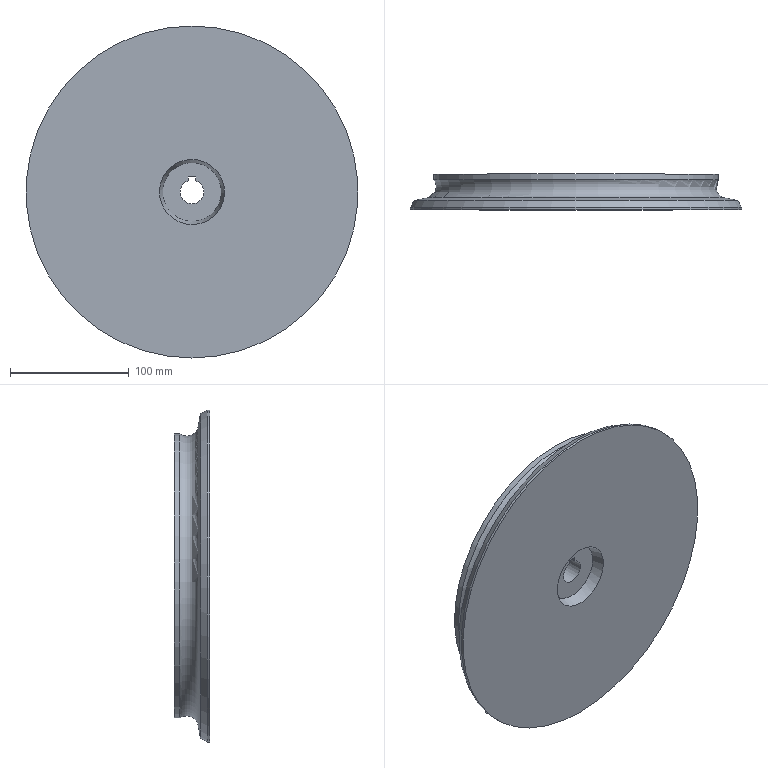Part | NX | features DATUM_CSYS 5, SKETCH 4, EXTRUDE 3, CPROJ 1, Delete Body 1, HOLE PACKAGE 1, SIMPLE HOLE 1, SWP104 1 | 1 solid | 13 faces | box 280 x 30 x 280 mm | volume 1461901 mm3 | plane 6 | cylinder 3 | cone 3 | torus 1 | commonest cylinder face diameters 20 x1 240.085 x1 280 x1
STEP:
#1=CARTESIAN_POINT('',(-3.,31.,151.135));
#2=VERTEX_POINT('',#1);
#3=CARTESIAN_POINT('',(-3.,31.,154.395));
#4=VERTEX_POINT('',#3);
#5=CARTESIAN_POINT('',(-3.,31.,141.595));
#6=DIRECTION('',(0.,0.,1.));
#7=VECTOR('',#6,1000.);
#8=LINE('',#5,#7);
#9=EDGE_CURVE('',#2,#4,#8,.T.);
#10=ORIENTED_EDGE('',*,*,#9,.F.);
#11=CARTESIAN_POINT('',(3.,31.,151.135));
#12=VERTEX_POINT('',#11);
#13=CARTESIAN_POINT('',(0.,31.,141.595));
#14=DIRECTION('',(0.,1.,0.));
#15=DIRECTION('',(0.,0.,1.));
#16=AXIS2_PLACEMENT_3D('',#13,#14,#15);
#17=CIRCLE('',#16,10.);
#18=EDGE_CURVE('',#12,#2,#17,.T.);
#19=ORIENTED_EDGE('',*,*,#18,.F.);
#20=CARTESIAN_POINT('',(3.,31.,154.395));
#21=VERTEX_POINT('',#20);
#22=CARTESIAN_POINT('',(3.,31.,141.595));
#23=DIRECTION('',(0.,0.,-1.));
#24=VECTOR('',#23,1000.);
#25=LINE('',#22,#24);
#26=EDGE_CURVE('',#21,#12,#25,.T.);
#27=ORIENTED_EDGE('',*,*,#26,.F.);
#28=CARTESIAN_POINT('',(0.,31.,154.395));
#29=DIRECTION('',(1.,0.,0.));
#30=VECTOR('',#29,1000.);
#31=LINE('',#28,#30);
#32=EDGE_CURVE('',#4,#21,#31,.T.);
#33=ORIENTED_EDGE('',*,*,#32,.F.);
#34=EDGE_LOOP('',(#10,#19,#27,#33));
#35=FACE_BOUND('',#34,.T.);
#36=CARTESIAN_POINT('',(0.,31.,261.638));
#37=VERTEX_POINT('',#36);
#38=CARTESIAN_POINT('',(0.,31.,141.595));
#39=DIRECTION('',(0.,1.,0.));
#40=DIRECTION('',(0.,0.,1.));
#41=AXIS2_PLACEMENT_3D('',#38,#39,#40);
#42=CIRCLE('',#41,120.043);
#43=EDGE_CURVE('',#37,#37,#42,.T.);
#44=ORIENTED_EDGE('',*,*,#43,.T.);
#45=EDGE_LOOP('',(#44));
#46=FACE_BOUND('',#45,.T.);
#47=CARTESIAN_POINT('',(0.,31.,141.595));
#48=DIRECTION('',(0.,1.,0.));
#49=DIRECTION('',(0.,0.,1.));
#50=AXIS2_PLACEMENT_3D('',#47,#48,#49);
#51=PLANE('',#50);
#52=ADVANCED_FACE('',(#35,#46),#51,.T.);
#53=CARTESIAN_POINT('',(27.473,1.,140.371));
#54=VERTEX_POINT('',#53);
#55=CARTESIAN_POINT('',(0.,1.,141.595));
#56=DIRECTION('',(0.,-1.,0.));
#57=DIRECTION('',(0.999,0.,-0.04452));
#58=AXIS2_PLACEMENT_3D('',#55,#56,#57);
#59=CIRCLE('',#58,27.5);
#60=EDGE_CURVE('',#54,#54,#59,.T.);
#61=ORIENTED_EDGE('',*,*,#60,.F.);
#62=EDGE_LOOP('',(#61));
#63=FACE_BOUND('',#62,.T.);
#64=CARTESIAN_POINT('',(0.,1.,281.595));
#65=VERTEX_POINT('',#64);
#66=CARTESIAN_POINT('',(0.,1.,141.595));
#67=DIRECTION('',(0.,1.,0.));
#68=DIRECTION('',(0.,0.,1.));
#69=AXIS2_PLACEMENT_3D('',#66,#67,#68);
#70=CIRCLE('',#69,140.);
#71=EDGE_CURVE('',#65,#65,#70,.T.);
#72=ORIENTED_EDGE('',*,*,#71,.F.);
#73=EDGE_LOOP('',(#72));
#74=FACE_BOUND('',#73,.T.);
#75=CARTESIAN_POINT('',(0.,1.,141.595));
#76=DIRECTION('',(0.,1.,0.));
#77=DIRECTION('',(0.,0.,1.));
#78=AXIS2_PLACEMENT_3D('',#75,#76,#77);
#79=PLANE('',#78);
#80=ADVANCED_FACE('',(#63,#74),#79,.F.);
#81=ORIENTED_EDGE('',*,*,#71,.T.);
#82=EDGE_LOOP('',(#81));
#83=FACE_BOUND('',#82,.T.);
#84=CARTESIAN_POINT('',(0.,3.,281.595));
#85=VERTEX_POINT('',#84);
#86=CARTESIAN_POINT('',(0.,3.,141.595));
#87=DIRECTION('',(0.,1.,0.));
#88=DIRECTION('',(0.,0.,1.));
#89=AXIS2_PLACEMENT_3D('',#86,#87,#88);
#90=CIRCLE('',#89,140.);
#91=EDGE_CURVE('',#85,#85,#90,.T.);
#92=ORIENTED_EDGE('',*,*,#91,.F.);
#93=EDGE_LOOP('',(#92));
#94=FACE_BOUND('',#93,.T.);
#95=CARTESIAN_POINT('',(0.,106.,141.595));
#96=DIRECTION('',(0.,1.,0.));
#97=DIRECTION('',(0.,0.,1.));
#98=AXIS2_PLACEMENT_3D('',#95,#96,#97);
#99=CYLINDRICAL_SURFACE('',#98,140.);
#100=ADVANCED_FACE('',(#83,#94),#99,.T.);
#101=ORIENTED_EDGE('',*,*,#91,.T.);
#102=EDGE_LOOP('',(#101));
#103=FACE_BOUND('',#102,.T.);
#104=CARTESIAN_POINT('',(0.,8.757,278.534));
#105=VERTEX_POINT('',#104);
#106=CARTESIAN_POINT('',(0.,8.757,141.595));
#107=DIRECTION('',(0.,1.,0.));
#108=DIRECTION('',(0.,0.,1.));
#109=AXIS2_PLACEMENT_3D('',#106,#107,#108);
#110=CIRCLE('',#109,136.939);
#111=EDGE_CURVE('',#105,#105,#110,.T.);
#112=ORIENTED_EDGE('',*,*,#111,.F.);
#113=EDGE_LOOP('',(#112));
#114=FACE_BOUND('',#113,.T.);
#115=CARTESIAN_POINT('',(0.,8.757,141.595));
#116=DIRECTION('',(0.,-1.,0.));
#117=DIRECTION('',(0.,0.,-1.));
#118=AXIS2_PLACEMENT_3D('',#115,#116,#117);
#119=CONICAL_SURFACE('',#118,136.939,0.4887);
#120=ADVANCED_FACE('',(#103,#114),#119,.T.);
#121=ORIENTED_EDGE('',*,*,#111,.T.);
#122=EDGE_LOOP('',(#121));
#123=FACE_BOUND('',#122,.T.);
#124=CARTESIAN_POINT('',(0.,10.917,267.422));
#125=VERTEX_POINT('',#124);
#126=CARTESIAN_POINT('',(0.,10.917,141.595));
#127=DIRECTION('',(0.,1.,0.));
#128=DIRECTION('',(0.,0.,1.));
#129=AXIS2_PLACEMENT_3D('',#126,#127,#128);
#130=CIRCLE('',#129,125.827);
#131=EDGE_CURVE('',#125,#125,#130,.T.);
#132=ORIENTED_EDGE('',*,*,#131,.F.);
#133=EDGE_LOOP('',(#132));
#134=FACE_BOUND('',#133,.T.);
#135=CARTESIAN_POINT('',(0.,10.917,141.595));
#136=DIRECTION('',(0.,-1.,0.));
#137=DIRECTION('',(0.,0.,-1.));
#138=AXIS2_PLACEMENT_3D('',#135,#136,#137);
#139=CONICAL_SURFACE('',#138,125.827,1.379);
#140=ADVANCED_FACE('',(#123,#134),#139,.T.);
#141=ORIENTED_EDGE('',*,*,#131,.T.);
#142=EDGE_LOOP('',(#141));
#143=FACE_BOUND('',#142,.T.);
#144=CARTESIAN_POINT('',(0.,26.232,261.638));
#145=VERTEX_POINT('',#144);
#146=CARTESIAN_POINT('',(0.,26.232,141.595));
#147=DIRECTION('',(0.,1.,0.));
#148=DIRECTION('',(0.,0.,1.));
#149=AXIS2_PLACEMENT_3D('',#146,#147,#148);
#150=CIRCLE('',#149,120.043);
#151=EDGE_CURVE('',#145,#145,#150,.T.);
#152=ORIENTED_EDGE('',*,*,#151,.F.);
#153=EDGE_LOOP('',(#152));
#154=FACE_BOUND('',#153,.T.);
#155=CARTESIAN_POINT('',(0.,20.36,141.595));
#156=DIRECTION('',(0.,1.,0.));
#157=DIRECTION('',(0.,0.,1.));
#158=AXIS2_PLACEMENT_3D('',#155,#156,#157);
#159=TOROIDAL_SURFACE('',#158,127.663,9.62);
#160=ADVANCED_FACE('',(#143,#154),#159,.F.);
#161=ORIENTED_EDGE('',*,*,#151,.T.);
#162=EDGE_LOOP('',(#161));
#163=FACE_BOUND('',#162,.T.);
#164=ORIENTED_EDGE('',*,*,#43,.F.);
#165=EDGE_LOOP('',(#164));
#166=FACE_BOUND('',#165,.T.);
#167=CARTESIAN_POINT('',(0.,106.,141.595));
#168=DIRECTION('',(0.,1.,0.));
#169=DIRECTION('',(0.,0.,1.));
#170=AXIS2_PLACEMENT_3D('',#167,#168,#169);
#171=CYLINDRICAL_SURFACE('',#170,120.043);
#172=ADVANCED_FACE('',(#163,#166),#171,.T.);
#173=CARTESIAN_POINT('',(0.,11.,116.775));
#174=VERTEX_POINT('',#173);
#175=CARTESIAN_POINT('',(0.,11.,141.595));
#176=DIRECTION('',(0.,-1.,0.));
#177=DIRECTION('',(0.,0.,-1.));
#178=AXIS2_PLACEMENT_3D('',#175,#176,#177);
#179=CIRCLE('',#178,24.821);
#180=EDGE_CURVE('',#174,#174,#179,.F.);
#181=ORIENTED_EDGE('',*,*,#180,.T.);
#182=EDGE_LOOP('',(#181));
#183=FACE_BOUND('',#182,.T.);
#184=ORIENTED_EDGE('',*,*,#60,.T.);
#185=EDGE_LOOP('',(#184));
#186=FACE_BOUND('',#185,.T.);
#187=CARTESIAN_POINT('',(0.,1.,141.595));
#188=DIRECTION('',(0.,-1.,0.));
#189=DIRECTION('',(0.999,0.,-0.04452));
#190=AXIS2_PLACEMENT_3D('',#187,#188,#189);
#191=CONICAL_SURFACE('',#190,27.5,0.2618);
#192=ADVANCED_FACE('',(#183,#186),#191,.F.);
#193=CARTESIAN_POINT('',(-3.,11.,154.395));
#194=VERTEX_POINT('',#193);
#195=CARTESIAN_POINT('',(-3.,11.,151.135));
#196=VERTEX_POINT('',#195);
#197=CARTESIAN_POINT('',(-3.,11.,154.395));
#198=DIRECTION('',(0.,0.,-1.));
#199=VECTOR('',#198,1000.);
#200=LINE('',#197,#199);
#201=EDGE_CURVE('',#194,#196,#200,.T.);
#202=ORIENTED_EDGE('',*,*,#201,.F.);
#203=CARTESIAN_POINT('',(3.,11.,154.395));
#204=VERTEX_POINT('',#203);
#205=CARTESIAN_POINT('',(3.,11.,154.395));
#206=DIRECTION('',(-1.,0.,0.));
#207=VECTOR('',#206,1000.);
#208=LINE('',#205,#207);
#209=EDGE_CURVE('',#204,#194,#208,.T.);
#210=ORIENTED_EDGE('',*,*,#209,.F.);
#211=CARTESIAN_POINT('',(3.,11.,151.135));
#212=VERTEX_POINT('',#211);
#213=CARTESIAN_POINT('',(3.,11.,141.595));
#214=DIRECTION('',(0.,0.,1.));
#215=VECTOR('',#214,1000.);
#216=LINE('',#213,#215);
#217=EDGE_CURVE('',#212,#204,#216,.T.);
#218=ORIENTED_EDGE('',*,*,#217,.F.);
#219=CARTESIAN_POINT('',(0.,11.,141.595));
#220=DIRECTION('',(0.,1.,0.));
#221=DIRECTION('',(0.,0.,1.));
#222=AXIS2_PLACEMENT_3D('',#219,#220,#221);
#223=CIRCLE('',#222,10.);
#224=EDGE_CURVE('',#212,#196,#223,.T.);
#225=ORIENTED_EDGE('',*,*,#224,.T.);
#226=EDGE_LOOP('',(#202,#210,#218,#225));
#227=FACE_BOUND('',#226,.T.);
#228=ORIENTED_EDGE('',*,*,#180,.F.);
#229=EDGE_LOOP('',(#228));
#230=FACE_BOUND('',#229,.T.);
#231=CARTESIAN_POINT('',(0.,11.,141.595));
#232=DIRECTION('',(0.,-1.,0.));
#233=DIRECTION('',(0.,0.,-1.));
#234=AXIS2_PLACEMENT_3D('',#231,#232,#233);
#235=PLANE('',#234);
#236=ADVANCED_FACE('',(#227,#230),#235,.T.);
#237=ORIENTED_EDGE('',*,*,#18,.T.);
#238=CARTESIAN_POINT('',(-3.,11.,151.135));
#239=DIRECTION('',(0.,1.,0.));
#240=VECTOR('',#239,1000.);
#241=LINE('',#238,#240);
#242=EDGE_CURVE('',#2,#196,#241,.F.);
#243=ORIENTED_EDGE('',*,*,#242,.T.);
#244=ORIENTED_EDGE('',*,*,#224,.F.);
#245=CARTESIAN_POINT('',(3.,11.,151.135));
#246=DIRECTION('',(0.,1.,0.));
#247=VECTOR('',#246,1000.);
#248=LINE('',#245,#247);
#249=EDGE_CURVE('',#212,#12,#248,.T.);
#250=ORIENTED_EDGE('',*,*,#249,.T.);
#251=EDGE_LOOP('',(#237,#243,#244,#250));
#252=FACE_BOUND('',#251,.T.);
#253=CARTESIAN_POINT('',(0.,11.,141.595));
#254=DIRECTION('',(0.,1.,0.));
#255=DIRECTION('',(0.,0.,1.));
#256=AXIS2_PLACEMENT_3D('',#253,#254,#255);
#257=CYLINDRICAL_SURFACE('',#256,10.);
#258=ADVANCED_FACE('',(#252),#257,.F.);
#259=ORIENTED_EDGE('',*,*,#9,.T.);
#260=CARTESIAN_POINT('',(-3.,33.,154.395));
#261=DIRECTION('',(0.,-1.,0.));
#262=VECTOR('',#261,1000.);
#263=LINE('',#260,#262);
#264=EDGE_CURVE('',#194,#4,#263,.F.);
#265=ORIENTED_EDGE('',*,*,#264,.F.);
#266=ORIENTED_EDGE('',*,*,#201,.T.);
#267=ORIENTED_EDGE('',*,*,#242,.F.);
#268=EDGE_LOOP('',(#259,#265,#266,#267));
#269=FACE_BOUND('',#268,.T.);
#270=CARTESIAN_POINT('',(-3.,33.,154.395));
#271=DIRECTION('',(-1.,0.,0.));
#272=DIRECTION('',(0.,0.,1.));
#273=AXIS2_PLACEMENT_3D('',#270,#271,#272);
#274=PLANE('',#273);
#275=ADVANCED_FACE('',(#269),#274,.F.);
#276=ORIENTED_EDGE('',*,*,#26,.T.);
#277=ORIENTED_EDGE('',*,*,#249,.F.);
#278=ORIENTED_EDGE('',*,*,#217,.T.);
#279=CARTESIAN_POINT('',(3.,33.,154.395));
#280=DIRECTION('',(0.,-1.,0.));
#281=VECTOR('',#280,1000.);
#282=LINE('',#279,#281);
#283=EDGE_CURVE('',#204,#21,#282,.F.);
#284=ORIENTED_EDGE('',*,*,#283,.T.);
#285=EDGE_LOOP('',(#276,#277,#278,#284));
#286=FACE_BOUND('',#285,.T.);
#287=CARTESIAN_POINT('',(3.,33.,141.595));
#288=DIRECTION('',(1.,0.,0.));
#289=DIRECTION('',(0.,0.,-1.));
#290=AXIS2_PLACEMENT_3D('',#287,#288,#289);
#291=PLANE('',#290);
#292=ADVANCED_FACE('',(#286),#291,.F.);
#293=ORIENTED_EDGE('',*,*,#32,.T.);
#294=ORIENTED_EDGE('',*,*,#283,.F.);
#295=ORIENTED_EDGE('',*,*,#209,.T.);
#296=ORIENTED_EDGE('',*,*,#264,.T.);
#297=EDGE_LOOP('',(#293,#294,#295,#296));
#298=FACE_BOUND('',#297,.T.);
#299=CARTESIAN_POINT('',(3.,33.,154.395));
#300=DIRECTION('',(0.,0.,1.));
#301=DIRECTION('',(1.,0.,0.));
#302=AXIS2_PLACEMENT_3D('',#299,#300,#301);
#303=PLANE('',#302);
#304=ADVANCED_FACE('',(#298),#303,.F.);
#305=CLOSED_SHELL('',(#52,#80,#100,#120,#140,#160,#172,#192,#236,#258,#275,#292,#304));
#306=MANIFOLD_SOLID_BREP('',#305);
#307=(LENGTH_UNIT()NAMED_UNIT(*)SI_UNIT(.MILLI.,.METRE.));
#308=UNCERTAINTY_MEASURE_WITH_UNIT(LENGTH_MEASURE(0.00001),#307,'','');
#309=(NAMED_UNIT(*)PLANE_ANGLE_UNIT()SI_UNIT($,.RADIAN.));
#310=(NAMED_UNIT(*)SI_UNIT($,.STERADIAN.)SOLID_ANGLE_UNIT());
#311=(GEOMETRIC_REPRESENTATION_CONTEXT(3)GLOBAL_UNCERTAINTY_ASSIGNED_CONTEXT((#308))GLOBAL_UNIT_ASSIGNED_CONTEXT((#307,#309,#310))REPRESENTATION_CONTEXT('',''));
#312=ADVANCED_BREP_SHAPE_REPRESENTATION('',(#306),#311);